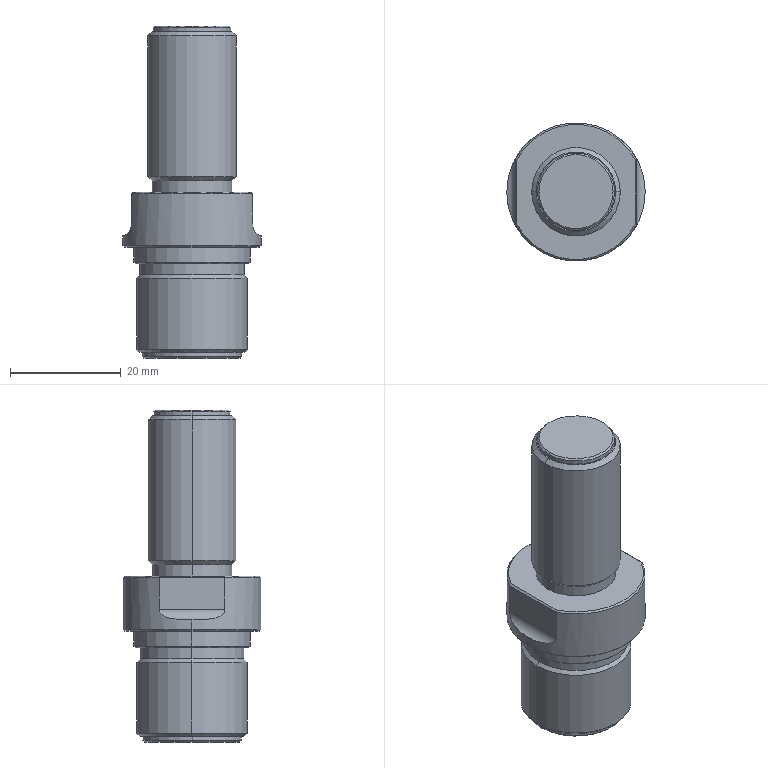Part | STEP file | 05螺纹接头 EDA50-L_R-005-BZ^EDA50-R04 (D60N) | 1 solid | 47 faces | box 25 x 25 x 60 mm | volume 16821 mm3 | cone 18 | cylinder 18 | plane 11 | commonest cylinder face diameters 4 x2 14 x2 14.4 x2 16 x2 18 x2 18.8 x2